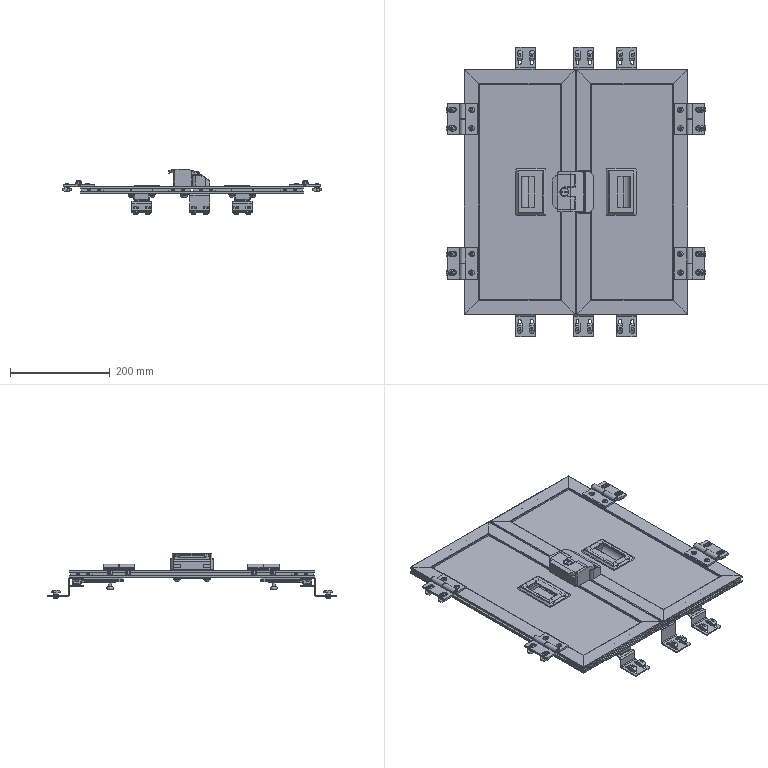Part | NX | features BREP 38 | 204 solids | 4860 faces | volume 1829823 mm3 | plane 2683 | cylinder 1481 | cone 560 | torus 102 | sphere 34 | commonest cylinder face diameters 5 x412 6 x114 4 x101 8 x96 1 x87 2 x73